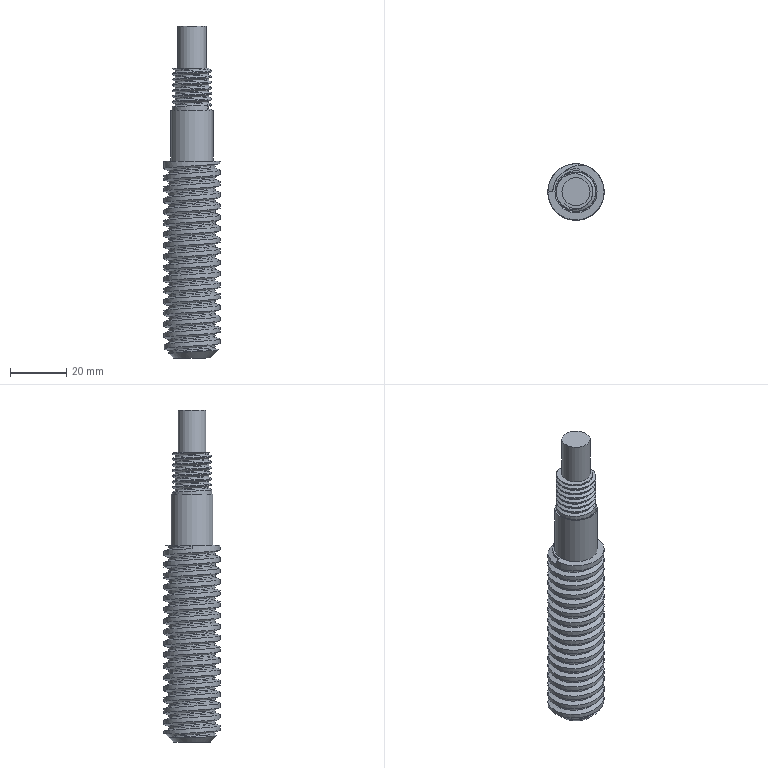Part | STEP file | YBQDJ-YL-11 | 1 solid | 21 faces | box 20 x 20 x 118 mm | volume 24858 mm3 | plane 8 | spline 7 | cylinder 5 | cone 1 | commonest cylinder face diameters 10 x1 12 x1 14 x1 15 x1 20 x1